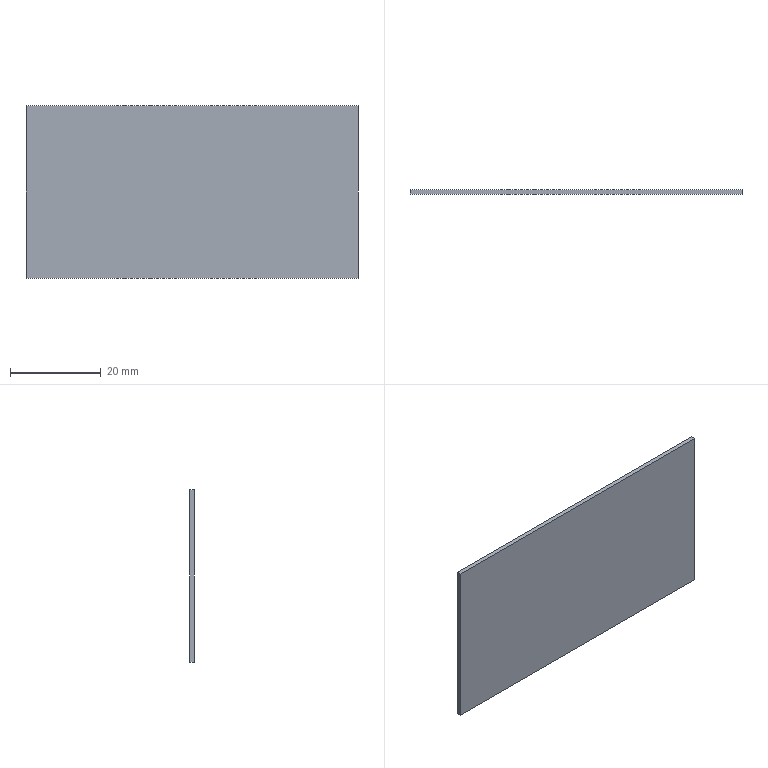Part | STEP file | 09-19 Outlet side seal plate 2 | 1 solid | 6 faces | box 73 x 1 x 38 mm | volume 2774 mm3 | plane 6
STEP:
#1=CARTESIAN_POINT('',(0.,0.,0.));
#2=DIRECTION('',(0.,0.,1.));
#3=DIRECTION('',(1.,0.,0.));
#4=AXIS2_PLACEMENT_3D('',#1,#2,#3);
#5=CARTESIAN_POINT('',(73.,0.,0.));
#6=VERTEX_POINT('',#5);
#7=CARTESIAN_POINT('',(0.,0.,0.));
#8=VERTEX_POINT('',#7);
#9=CARTESIAN_POINT('',(36.5,0.,0.));
#10=DIRECTION('',(-1.,0.,0.));
#11=VECTOR('',#10,1.);
#12=LINE('',#9,#11);
#13=CARTESIAN_POINT('',(73.,0.,0.));
#14=DIRECTION('',(0.,0.,-1.));
#15=DIRECTION('',(-1.,0.,0.));
#16=AXIS2_PLACEMENT_3D('',#13,#14,#15);
#17=PLANE('',#16);
#18=CARTESIAN_POINT('',(36.5,0.));
#19=DIRECTION('',(1.,0.));
#20=VECTOR('',#19,1.);
#21=LINE('',#18,#20);
#22=(GEOMETRIC_REPRESENTATION_CONTEXT(2)PARAMETRIC_REPRESENTATION_CONTEXT()REPRESENTATION_CONTEXT('',''));
#23=DEFINITIONAL_REPRESENTATION('',(#21),#22);
#24=PCURVE('',#17,#23);
#25=CARTESIAN_POINT('',(0.,0.,-38.));
#26=DIRECTION('',(0.,1.,0.));
#27=DIRECTION('',(0.,0.,1.));
#28=AXIS2_PLACEMENT_3D('',#25,#26,#27);
#29=PLANE('',#28);
#30=CARTESIAN_POINT('',(38.,36.5));
#31=DIRECTION('',(0.,-1.));
#32=VECTOR('',#31,1.);
#33=LINE('',#30,#32);
#34=(GEOMETRIC_REPRESENTATION_CONTEXT(2)PARAMETRIC_REPRESENTATION_CONTEXT()REPRESENTATION_CONTEXT('',''));
#35=DEFINITIONAL_REPRESENTATION('',(#33),#34);
#36=PCURVE('',#29,#35);
#37=SURFACE_CURVE('',#12,(#24,#36),.PCURVE_S1.);
#38=EDGE_CURVE('',#6,#8,#37,.T.);
#39=ORIENTED_EDGE('',*,*,#38,.F.);
#40=CARTESIAN_POINT('',(73.,1.,0.));
#41=VERTEX_POINT('',#40);
#42=CARTESIAN_POINT('',(73.,0.5,0.));
#43=DIRECTION('',(0.,1.,0.));
#44=VECTOR('',#43,1.);
#45=LINE('',#42,#44);
#46=CARTESIAN_POINT('',(0.,0.5));
#47=DIRECTION('',(0.,1.));
#48=VECTOR('',#47,1.);
#49=LINE('',#46,#48);
#50=(GEOMETRIC_REPRESENTATION_CONTEXT(2)PARAMETRIC_REPRESENTATION_CONTEXT()REPRESENTATION_CONTEXT('',''));
#51=DEFINITIONAL_REPRESENTATION('',(#49),#50);
#52=PCURVE('',#17,#51);
#53=CARTESIAN_POINT('',(73.,0.,-38.));
#54=DIRECTION('',(-1.,0.,0.));
#55=DIRECTION('',(0.,0.,1.));
#56=AXIS2_PLACEMENT_3D('',#53,#54,#55);
#57=PLANE('',#56);
#58=CARTESIAN_POINT('',(38.,0.5));
#59=DIRECTION('',(0.,1.));
#60=VECTOR('',#59,1.);
#61=LINE('',#58,#60);
#62=(GEOMETRIC_REPRESENTATION_CONTEXT(2)PARAMETRIC_REPRESENTATION_CONTEXT()REPRESENTATION_CONTEXT('',''));
#63=DEFINITIONAL_REPRESENTATION('',(#61),#62);
#64=PCURVE('',#57,#63);
#65=SURFACE_CURVE('',#45,(#52,#64),.PCURVE_S1.);
#66=EDGE_CURVE('',#6,#41,#65,.T.);
#67=ORIENTED_EDGE('',*,*,#66,.T.);
#68=CARTESIAN_POINT('',(0.,1.,0.));
#69=VERTEX_POINT('',#68);
#70=CARTESIAN_POINT('',(36.5,1.,0.));
#71=DIRECTION('',(1.,0.,0.));
#72=VECTOR('',#71,1.);
#73=LINE('',#70,#72);
#74=CARTESIAN_POINT('',(36.5,1.));
#75=DIRECTION('',(-1.,0.));
#76=VECTOR('',#75,1.);
#77=LINE('',#74,#76);
#78=(GEOMETRIC_REPRESENTATION_CONTEXT(2)PARAMETRIC_REPRESENTATION_CONTEXT()REPRESENTATION_CONTEXT('',''));
#79=DEFINITIONAL_REPRESENTATION('',(#77),#78);
#80=PCURVE('',#17,#79);
#81=CARTESIAN_POINT('',(0.,1.,0.));
#82=DIRECTION('',(0.,-1.,0.));
#83=DIRECTION('',(0.,0.,-1.));
#84=AXIS2_PLACEMENT_3D('',#81,#82,#83);
#85=PLANE('',#84);
#86=CARTESIAN_POINT('',(0.,36.5));
#87=DIRECTION('',(0.,1.));
#88=VECTOR('',#87,1.);
#89=LINE('',#86,#88);
#90=(GEOMETRIC_REPRESENTATION_CONTEXT(2)PARAMETRIC_REPRESENTATION_CONTEXT()REPRESENTATION_CONTEXT('',''));
#91=DEFINITIONAL_REPRESENTATION('',(#89),#90);
#92=PCURVE('',#85,#91);
#93=SURFACE_CURVE('',#73,(#80,#92),.PCURVE_S1.);
#94=EDGE_CURVE('',#69,#41,#93,.T.);
#95=ORIENTED_EDGE('',*,*,#94,.F.);
#96=CARTESIAN_POINT('',(0.,0.5,0.));
#97=DIRECTION('',(0.,1.,0.));
#98=VECTOR('',#97,1.);
#99=LINE('',#96,#98);
#100=CARTESIAN_POINT('',(73.,0.5));
#101=DIRECTION('',(0.,1.));
#102=VECTOR('',#101,1.);
#103=LINE('',#100,#102);
#104=(GEOMETRIC_REPRESENTATION_CONTEXT(2)PARAMETRIC_REPRESENTATION_CONTEXT()REPRESENTATION_CONTEXT('',''));
#105=DEFINITIONAL_REPRESENTATION('',(#103),#104);
#106=PCURVE('',#17,#105);
#107=CARTESIAN_POINT('',(0.,0.,-38.));
#108=DIRECTION('',(-1.,0.,0.));
#109=DIRECTION('',(0.,0.,1.));
#110=AXIS2_PLACEMENT_3D('',#107,#108,#109);
#111=PLANE('',#110);
#112=CARTESIAN_POINT('',(38.,0.5));
#113=DIRECTION('',(0.,1.));
#114=VECTOR('',#113,1.);
#115=LINE('',#112,#114);
#116=(GEOMETRIC_REPRESENTATION_CONTEXT(2)PARAMETRIC_REPRESENTATION_CONTEXT()REPRESENTATION_CONTEXT('',''));
#117=DEFINITIONAL_REPRESENTATION('',(#115),#116);
#118=PCURVE('',#111,#117);
#119=SURFACE_CURVE('',#99,(#106,#118),.PCURVE_S1.);
#120=EDGE_CURVE('',#8,#69,#119,.T.);
#121=ORIENTED_EDGE('',*,*,#120,.F.);
#122=EDGE_LOOP('',(#39,#67,#95,#121));
#123=FACE_BOUND('',#122,.T.);
#124=ADVANCED_FACE('',(#123),#17,.F.);
#125=CARTESIAN_POINT('',(73.,0.,-38.));
#126=VERTEX_POINT('',#125);
#127=CARTESIAN_POINT('',(0.,0.,-38.));
#128=VERTEX_POINT('',#127);
#129=CARTESIAN_POINT('',(36.5,0.,-38.));
#130=DIRECTION('',(-1.,0.,0.));
#131=VECTOR('',#130,1.);
#132=LINE('',#129,#131);
#133=CARTESIAN_POINT('',(0.,36.5));
#134=DIRECTION('',(0.,-1.));
#135=VECTOR('',#134,1.);
#136=LINE('',#133,#135);
#137=(GEOMETRIC_REPRESENTATION_CONTEXT(2)PARAMETRIC_REPRESENTATION_CONTEXT()REPRESENTATION_CONTEXT('',''));
#138=DEFINITIONAL_REPRESENTATION('',(#136),#137);
#139=PCURVE('',#29,#138);
#140=CARTESIAN_POINT('',(0.,0.,-38.));
#141=DIRECTION('',(0.,0.,1.));
#142=DIRECTION('',(1.,0.,0.));
#143=AXIS2_PLACEMENT_3D('',#140,#141,#142);
#144=PLANE('',#143);
#145=CARTESIAN_POINT('',(36.5,0.));
#146=DIRECTION('',(-1.,0.));
#147=VECTOR('',#146,1.);
#148=LINE('',#145,#147);
#149=(GEOMETRIC_REPRESENTATION_CONTEXT(2)PARAMETRIC_REPRESENTATION_CONTEXT()REPRESENTATION_CONTEXT('',''));
#150=DEFINITIONAL_REPRESENTATION('',(#148),#149);
#151=PCURVE('',#144,#150);
#152=SURFACE_CURVE('',#132,(#139,#151),.PCURVE_S1.);
#153=EDGE_CURVE('',#126,#128,#152,.T.);
#154=ORIENTED_EDGE('',*,*,#153,.F.);
#155=CARTESIAN_POINT('',(73.,0.,-19.));
#156=DIRECTION('',(0.,0.,-1.));
#157=VECTOR('',#156,1.);
#158=LINE('',#155,#157);
#159=CARTESIAN_POINT('',(19.,73.));
#160=DIRECTION('',(-1.,0.));
#161=VECTOR('',#160,1.);
#162=LINE('',#159,#161);
#163=(GEOMETRIC_REPRESENTATION_CONTEXT(2)PARAMETRIC_REPRESENTATION_CONTEXT()REPRESENTATION_CONTEXT('',''));
#164=DEFINITIONAL_REPRESENTATION('',(#162),#163);
#165=PCURVE('',#29,#164);
#166=CARTESIAN_POINT('',(19.,0.));
#167=DIRECTION('',(-1.,0.));
#168=VECTOR('',#167,1.);
#169=LINE('',#166,#168);
#170=(GEOMETRIC_REPRESENTATION_CONTEXT(2)PARAMETRIC_REPRESENTATION_CONTEXT()REPRESENTATION_CONTEXT('',''));
#171=DEFINITIONAL_REPRESENTATION('',(#169),#170);
#172=PCURVE('',#57,#171);
#173=SURFACE_CURVE('',#158,(#165,#172),.PCURVE_S1.);
#174=EDGE_CURVE('',#6,#126,#173,.T.);
#175=ORIENTED_EDGE('',*,*,#174,.F.);
#176=ORIENTED_EDGE('',*,*,#38,.T.);
#177=CARTESIAN_POINT('',(0.,0.,-19.));
#178=DIRECTION('',(0.,0.,1.));
#179=VECTOR('',#178,1.);
#180=LINE('',#177,#179);
#181=CARTESIAN_POINT('',(19.,0.));
#182=DIRECTION('',(1.,0.));
#183=VECTOR('',#182,1.);
#184=LINE('',#181,#183);
#185=(GEOMETRIC_REPRESENTATION_CONTEXT(2)PARAMETRIC_REPRESENTATION_CONTEXT()REPRESENTATION_CONTEXT('',''));
#186=DEFINITIONAL_REPRESENTATION('',(#184),#185);
#187=PCURVE('',#29,#186);
#188=CARTESIAN_POINT('',(19.,0.));
#189=DIRECTION('',(1.,0.));
#190=VECTOR('',#189,1.);
#191=LINE('',#188,#190);
#192=(GEOMETRIC_REPRESENTATION_CONTEXT(2)PARAMETRIC_REPRESENTATION_CONTEXT()REPRESENTATION_CONTEXT('',''));
#193=DEFINITIONAL_REPRESENTATION('',(#191),#192);
#194=PCURVE('',#111,#193);
#195=SURFACE_CURVE('',#180,(#187,#194),.PCURVE_S1.);
#196=EDGE_CURVE('',#128,#8,#195,.T.);
#197=ORIENTED_EDGE('',*,*,#196,.F.);
#198=EDGE_LOOP('',(#154,#175,#176,#197));
#199=FACE_BOUND('',#198,.T.);
#200=ADVANCED_FACE('',(#199),#29,.F.);
#201=ORIENTED_EDGE('',*,*,#94,.T.);
#202=CARTESIAN_POINT('',(73.,1.,-38.));
#203=VERTEX_POINT('',#202);
#204=CARTESIAN_POINT('',(73.,1.,-19.));
#205=DIRECTION('',(0.,0.,1.));
#206=VECTOR('',#205,1.);
#207=LINE('',#204,#206);
#208=CARTESIAN_POINT('',(19.,73.));
#209=DIRECTION('',(-1.,0.));
#210=VECTOR('',#209,1.);
#211=LINE('',#208,#210);
#212=(GEOMETRIC_REPRESENTATION_CONTEXT(2)PARAMETRIC_REPRESENTATION_CONTEXT()REPRESENTATION_CONTEXT('',''));
#213=DEFINITIONAL_REPRESENTATION('',(#211),#212);
#214=PCURVE('',#85,#213);
#215=CARTESIAN_POINT('',(19.,1.));
#216=DIRECTION('',(1.,0.));
#217=VECTOR('',#216,1.);
#218=LINE('',#215,#217);
#219=(GEOMETRIC_REPRESENTATION_CONTEXT(2)PARAMETRIC_REPRESENTATION_CONTEXT()REPRESENTATION_CONTEXT('',''));
#220=DEFINITIONAL_REPRESENTATION('',(#218),#219);
#221=PCURVE('',#57,#220);
#222=SURFACE_CURVE('',#207,(#214,#221),.PCURVE_S1.);
#223=EDGE_CURVE('',#203,#41,#222,.T.);
#224=ORIENTED_EDGE('',*,*,#223,.F.);
#225=CARTESIAN_POINT('',(0.,1.,-38.));
#226=VERTEX_POINT('',#225);
#227=CARTESIAN_POINT('',(36.5,1.,-38.));
#228=DIRECTION('',(1.,0.,0.));
#229=VECTOR('',#228,1.);
#230=LINE('',#227,#229);
#231=CARTESIAN_POINT('',(38.,36.5));
#232=DIRECTION('',(0.,1.));
#233=VECTOR('',#232,1.);
#234=LINE('',#231,#233);
#235=(GEOMETRIC_REPRESENTATION_CONTEXT(2)PARAMETRIC_REPRESENTATION_CONTEXT()REPRESENTATION_CONTEXT('',''));
#236=DEFINITIONAL_REPRESENTATION('',(#234),#235);
#237=PCURVE('',#85,#236);
#238=CARTESIAN_POINT('',(36.5,1.));
#239=DIRECTION('',(1.,0.));
#240=VECTOR('',#239,1.);
#241=LINE('',#238,#240);
#242=(GEOMETRIC_REPRESENTATION_CONTEXT(2)PARAMETRIC_REPRESENTATION_CONTEXT()REPRESENTATION_CONTEXT('',''));
#243=DEFINITIONAL_REPRESENTATION('',(#241),#242);
#244=PCURVE('',#144,#243);
#245=SURFACE_CURVE('',#230,(#237,#244),.PCURVE_S1.);
#246=EDGE_CURVE('',#226,#203,#245,.T.);
#247=ORIENTED_EDGE('',*,*,#246,.F.);
#248=CARTESIAN_POINT('',(0.,1.,-19.));
#249=DIRECTION('',(0.,0.,-1.));
#250=VECTOR('',#249,1.);
#251=LINE('',#248,#250);
#252=CARTESIAN_POINT('',(19.,0.));
#253=DIRECTION('',(1.,0.));
#254=VECTOR('',#253,1.);
#255=LINE('',#252,#254);
#256=(GEOMETRIC_REPRESENTATION_CONTEXT(2)PARAMETRIC_REPRESENTATION_CONTEXT()REPRESENTATION_CONTEXT('',''));
#257=DEFINITIONAL_REPRESENTATION('',(#255),#256);
#258=PCURVE('',#85,#257);
#259=CARTESIAN_POINT('',(19.,1.));
#260=DIRECTION('',(-1.,0.));
#261=VECTOR('',#260,1.);
#262=LINE('',#259,#261);
#263=(GEOMETRIC_REPRESENTATION_CONTEXT(2)PARAMETRIC_REPRESENTATION_CONTEXT()REPRESENTATION_CONTEXT('',''));
#264=DEFINITIONAL_REPRESENTATION('',(#262),#263);
#265=PCURVE('',#111,#264);
#266=SURFACE_CURVE('',#251,(#258,#265),.PCURVE_S1.);
#267=EDGE_CURVE('',#69,#226,#266,.T.);
#268=ORIENTED_EDGE('',*,*,#267,.F.);
#269=EDGE_LOOP('',(#201,#224,#247,#268));
#270=FACE_BOUND('',#269,.T.);
#271=ADVANCED_FACE('',(#270),#85,.F.);
#272=CARTESIAN_POINT('',(0.,0.5,-38.));
#273=DIRECTION('',(0.,-1.,0.));
#274=VECTOR('',#273,1.);
#275=LINE('',#272,#274);
#276=CARTESIAN_POINT('',(0.,0.5));
#277=DIRECTION('',(0.,-1.));
#278=VECTOR('',#277,1.);
#279=LINE('',#276,#278);
#280=(GEOMETRIC_REPRESENTATION_CONTEXT(2)PARAMETRIC_REPRESENTATION_CONTEXT()REPRESENTATION_CONTEXT('',''));
#281=DEFINITIONAL_REPRESENTATION('',(#279),#280);
#282=PCURVE('',#111,#281);
#283=CARTESIAN_POINT('',(0.,0.5));
#284=DIRECTION('',(0.,-1.));
#285=VECTOR('',#284,1.);
#286=LINE('',#283,#285);
#287=(GEOMETRIC_REPRESENTATION_CONTEXT(2)PARAMETRIC_REPRESENTATION_CONTEXT()REPRESENTATION_CONTEXT('',''));
#288=DEFINITIONAL_REPRESENTATION('',(#286),#287);
#289=PCURVE('',#144,#288);
#290=SURFACE_CURVE('',#275,(#282,#289),.PCURVE_S1.);
#291=EDGE_CURVE('',#226,#128,#290,.T.);
#292=ORIENTED_EDGE('',*,*,#291,.T.);
#293=ORIENTED_EDGE('',*,*,#196,.T.);
#294=ORIENTED_EDGE('',*,*,#120,.T.);
#295=ORIENTED_EDGE('',*,*,#267,.T.);
#296=EDGE_LOOP('',(#292,#293,#294,#295));
#297=FACE_BOUND('',#296,.T.);
#298=ADVANCED_FACE('',(#297),#111,.T.);
#299=ORIENTED_EDGE('',*,*,#246,.T.);
#300=CARTESIAN_POINT('',(73.,0.5,-38.));
#301=DIRECTION('',(0.,1.,0.));
#302=VECTOR('',#301,1.);
#303=LINE('',#300,#302);
#304=CARTESIAN_POINT('',(73.,0.5));
#305=DIRECTION('',(0.,1.));
#306=VECTOR('',#305,1.);
#307=LINE('',#304,#306);
#308=(GEOMETRIC_REPRESENTATION_CONTEXT(2)PARAMETRIC_REPRESENTATION_CONTEXT()REPRESENTATION_CONTEXT('',''));
#309=DEFINITIONAL_REPRESENTATION('',(#307),#308);
#310=PCURVE('',#144,#309);
#311=CARTESIAN_POINT('',(0.,0.5));
#312=DIRECTION('',(0.,1.));
#313=VECTOR('',#312,1.);
#314=LINE('',#311,#313);
#315=(GEOMETRIC_REPRESENTATION_CONTEXT(2)PARAMETRIC_REPRESENTATION_CONTEXT()REPRESENTATION_CONTEXT('',''));
#316=DEFINITIONAL_REPRESENTATION('',(#314),#315);
#317=PCURVE('',#57,#316);
#318=SURFACE_CURVE('',#303,(#310,#317),.PCURVE_S1.);
#319=EDGE_CURVE('',#126,#203,#318,.T.);
#320=ORIENTED_EDGE('',*,*,#319,.F.);
#321=ORIENTED_EDGE('',*,*,#153,.T.);
#322=ORIENTED_EDGE('',*,*,#291,.F.);
#323=EDGE_LOOP('',(#299,#320,#321,#322));
#324=FACE_BOUND('',#323,.T.);
#325=ADVANCED_FACE('',(#324),#144,.F.);
#326=ORIENTED_EDGE('',*,*,#174,.T.);
#327=ORIENTED_EDGE('',*,*,#319,.T.);
#328=ORIENTED_EDGE('',*,*,#223,.T.);
#329=ORIENTED_EDGE('',*,*,#66,.F.);
#330=EDGE_LOOP('',(#326,#327,#328,#329));
#331=FACE_BOUND('',#330,.T.);
#332=ADVANCED_FACE('',(#331),#57,.F.);
#333=CLOSED_SHELL('',(#124,#200,#271,#298,#325,#332));
#334=MANIFOLD_SOLID_BREP('',#333);
#335=(LENGTH_UNIT()NAMED_UNIT(*)SI_UNIT(.MILLI.,.METRE.));
#336=UNCERTAINTY_MEASURE_WITH_UNIT(LENGTH_MEASURE(0.0000001),#335,'','');
#337=(NAMED_UNIT(*)PLANE_ANGLE_UNIT()SI_UNIT($,.RADIAN.));
#338=(NAMED_UNIT(*)SI_UNIT($,.STERADIAN.)SOLID_ANGLE_UNIT());
#339=(GEOMETRIC_REPRESENTATION_CONTEXT(3)GLOBAL_UNCERTAINTY_ASSIGNED_CONTEXT((#336))GLOBAL_UNIT_ASSIGNED_CONTEXT((#335,#337,#338))REPRESENTATION_CONTEXT('',''));
#340=ADVANCED_BREP_SHAPE_REPRESENTATION('',(#4,#334),#339);